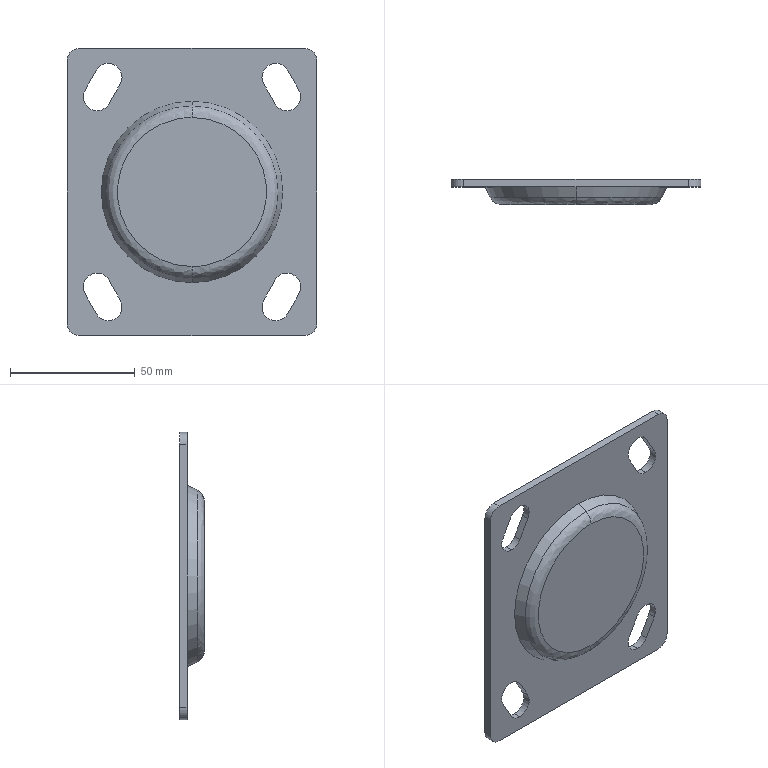Part | STEP file | _CEL21-100-P-002 | 1 solid | 41 faces | box 100 x 10 x 115 mm | volume 55123 mm3 | cylinder 20 | plane 17 | spline 2 | cone 2 | commonest cylinder face diameters 11 x12 10 x4 25 x2 66.667 x2
STEP:
#1=CARTESIAN_POINT('',(0.,84.,-60.815));
#2=VERTEX_POINT('',#1);
#3=CARTESIAN_POINT('',(0.,84.,-1.185));
#4=VERTEX_POINT('',#3);
#5=CARTESIAN_POINT('',(0.,84.,-60.815));
#6=CARTESIAN_POINT('',(-59.629,84.,-60.815));
#7=CARTESIAN_POINT('',(-59.629,84.,-1.185));
#8=CARTESIAN_POINT('',(0.,84.,-1.185));
#9=(BOUNDED_CURVE()B_SPLINE_CURVE(3,(#5,#6,#7,#8),.UNSPECIFIED.,.F.,.F.)B_SPLINE_CURVE_WITH_KNOTS((4,4),(0.,0.5),.UNSPECIFIED.)CURVE()GEOMETRIC_REPRESENTATION_ITEM()RATIONAL_B_SPLINE_CURVE((1.,0.3333,0.3333,1.))REPRESENTATION_ITEM(''));
#10=EDGE_CURVE('',#2,#4,#9,.T.);
#11=ORIENTED_EDGE('',*,*,#10,.T.);
#12=CARTESIAN_POINT('',(0.,86.887,3.346));
#13=VERTEX_POINT('',#12);
#14=CARTESIAN_POINT('',(0.,89.,-1.185));
#15=DIRECTION('',(-1.,0.,0.));
#16=DIRECTION('',(0.,0.,1.));
#17=AXIS2_PLACEMENT_3D('',#14,#15,#16);
#18=CIRCLE('',#17,5.);
#19=EDGE_CURVE('',#4,#13,#18,.T.);
#20=ORIENTED_EDGE('',*,*,#19,.T.);
#21=CARTESIAN_POINT('',(0.,86.887,-65.346));
#22=VERTEX_POINT('',#21);
#23=CARTESIAN_POINT('',(0.,86.887,-31.));
#24=DIRECTION('',(0.,1.,0.));
#25=DIRECTION('',(0.,0.,1.));
#26=AXIS2_PLACEMENT_3D('',#23,#24,#25);
#27=CIRCLE('',#26,34.346);
#28=EDGE_CURVE('',#22,#13,#27,.T.);
#29=ORIENTED_EDGE('',*,*,#28,.F.);
#30=CARTESIAN_POINT('',(0.,89.,-60.815));
#31=DIRECTION('',(1.,0.,0.));
#32=DIRECTION('',(0.,0.,-1.));
#33=AXIS2_PLACEMENT_3D('',#30,#31,#32);
#34=CIRCLE('',#33,5.);
#35=EDGE_CURVE('',#2,#22,#34,.T.);
#36=ORIENTED_EDGE('',*,*,#35,.F.);
#37=EDGE_LOOP('',(#11,#20,#29,#36));
#38=FACE_OUTER_BOUND('',#37,.T.);
#39=CARTESIAN_POINT('',(0.,84.,-1.185));
#40=CARTESIAN_POINT('',(-59.629,84.,-1.185));
#41=CARTESIAN_POINT('',(-59.629,84.,-60.815));
#42=CARTESIAN_POINT('',(0.,84.,-60.815));
#43=CARTESIAN_POINT('',(0.,84.,0.8144));
#44=CARTESIAN_POINT('',(-63.629,84.,0.8144));
#45=CARTESIAN_POINT('',(-63.629,84.,-62.814));
#46=CARTESIAN_POINT('',(0.,84.,-62.814));
#47=CARTESIAN_POINT('',(0.,85.074,2.501));
#48=CARTESIAN_POINT('',(-67.002,85.074,2.501));
#49=CARTESIAN_POINT('',(-67.002,85.074,-64.501));
#50=CARTESIAN_POINT('',(0.,85.074,-64.501));
#51=CARTESIAN_POINT('',(0.,86.887,3.346));
#52=CARTESIAN_POINT('',(-68.692,86.887,3.346));
#53=CARTESIAN_POINT('',(-68.692,86.887,-65.346));
#54=CARTESIAN_POINT('',(0.,86.887,-65.346));
#55=(BOUNDED_SURFACE()B_SPLINE_SURFACE(3,3,((#39,#40,#41,#42),(#43,#44,#45,#46),(#47,#48,#49,#50),(#51,#52,#53,#54)),.UNSPECIFIED.,.F.,.F.,.F.)B_SPLINE_SURFACE_WITH_KNOTS((4,4),(4,4),(0.,1.),(0.,1.),.UNSPECIFIED.)GEOMETRIC_REPRESENTATION_ITEM()RATIONAL_B_SPLINE_SURFACE(((1.,0.3333,0.3333,1.),(0.8956,0.2985,0.2985,0.8956),(0.8956,0.2985,0.2985,0.8956),(1.,0.3333,0.3333,1.)))REPRESENTATION_ITEM('')SURFACE());
#56=ADVANCED_FACE('',(#38),#55,.T.);
#57=CARTESIAN_POINT('',(33.5,94.,-82.5));
#58=VERTEX_POINT('',#57);
#59=CARTESIAN_POINT('',(38.294,94.,-79.696));
#60=VERTEX_POINT('',#59);
#61=CARTESIAN_POINT('',(33.5,94.,-77.));
#62=DIRECTION('',(0.,-1.,0.));
#63=DIRECTION('',(0.,0.,-1.));
#64=AXIS2_PLACEMENT_3D('',#61,#62,#63);
#65=CIRCLE('',#64,5.5);
#66=EDGE_CURVE('',#58,#60,#65,.T.);
#67=ORIENTED_EDGE('',*,*,#66,.F.);
#68=CARTESIAN_POINT('',(33.5,91.,-82.5));
#69=VERTEX_POINT('',#68);
#70=CARTESIAN_POINT('',(33.5,91.,-82.5));
#71=DIRECTION('',(0.,-1.,0.));
#72=VECTOR('',#71,1000.);
#73=LINE('',#70,#72);
#74=EDGE_CURVE('',#58,#69,#73,.T.);
#75=ORIENTED_EDGE('',*,*,#74,.T.);
#76=CARTESIAN_POINT('',(38.294,91.,-79.696));
#77=VERTEX_POINT('',#76);
#78=CARTESIAN_POINT('',(33.5,91.,-77.));
#79=DIRECTION('',(0.,1.,0.));
#80=DIRECTION('',(0.,0.,-1.));
#81=AXIS2_PLACEMENT_3D('',#78,#79,#80);
#82=CIRCLE('',#81,5.5);
#83=EDGE_CURVE('',#77,#69,#82,.T.);
#84=ORIENTED_EDGE('',*,*,#83,.F.);
#85=CARTESIAN_POINT('',(38.294,91.,-79.696));
#86=DIRECTION('',(0.,-1.,0.));
#87=VECTOR('',#86,1000.);
#88=LINE('',#85,#87);
#89=EDGE_CURVE('',#60,#77,#88,.T.);
#90=ORIENTED_EDGE('',*,*,#89,.F.);
#91=EDGE_LOOP('',(#67,#75,#84,#90));
#92=FACE_OUTER_BOUND('',#91,.T.);
#93=CARTESIAN_POINT('',(33.5,91.,-77.));
#94=DIRECTION('',(0.,-1.,0.));
#95=DIRECTION('',(0.,0.,-1.));
#96=AXIS2_PLACEMENT_3D('',#93,#94,#95);
#97=CYLINDRICAL_SURFACE('',#96,5.5);
#98=ADVANCED_FACE('',(#92),#97,.F.);
#99=CARTESIAN_POINT('',(38.,94.,1.5));
#100=VERTEX_POINT('',#99);
#101=CARTESIAN_POINT('',(42.794,94.,9.696));
#102=VERTEX_POINT('',#101);
#103=CARTESIAN_POINT('',(38.,94.,7.));
#104=DIRECTION('',(0.,-1.,0.));
#105=DIRECTION('',(0.,0.,-1.));
#106=AXIS2_PLACEMENT_3D('',#103,#104,#105);
#107=CIRCLE('',#106,5.5);
#108=EDGE_CURVE('',#100,#102,#107,.T.);
#109=ORIENTED_EDGE('',*,*,#108,.F.);
#110=CARTESIAN_POINT('',(38.,91.,1.5));
#111=VERTEX_POINT('',#110);
#112=CARTESIAN_POINT('',(38.,91.,1.5));
#113=DIRECTION('',(0.,-1.,0.));
#114=VECTOR('',#113,1000.);
#115=LINE('',#112,#114);
#116=EDGE_CURVE('',#100,#111,#115,.T.);
#117=ORIENTED_EDGE('',*,*,#116,.T.);
#118=CARTESIAN_POINT('',(42.794,91.,9.696));
#119=VERTEX_POINT('',#118);
#120=CARTESIAN_POINT('',(38.,91.,7.));
#121=DIRECTION('',(0.,1.,0.));
#122=DIRECTION('',(0.,0.,-1.));
#123=AXIS2_PLACEMENT_3D('',#120,#121,#122);
#124=CIRCLE('',#123,5.5);
#125=EDGE_CURVE('',#119,#111,#124,.T.);
#126=ORIENTED_EDGE('',*,*,#125,.F.);
#127=CARTESIAN_POINT('',(42.794,91.,9.696));
#128=DIRECTION('',(0.,1.,0.));
#129=VECTOR('',#128,1000.);
#130=LINE('',#127,#129);
#131=EDGE_CURVE('',#119,#102,#130,.T.);
#132=ORIENTED_EDGE('',*,*,#131,.T.);
#133=EDGE_LOOP('',(#109,#117,#126,#132));
#134=FACE_OUTER_BOUND('',#133,.T.);
#135=CARTESIAN_POINT('',(38.,91.,7.));
#136=DIRECTION('',(0.,-1.,0.));
#137=DIRECTION('',(0.,0.,-1.));
#138=AXIS2_PLACEMENT_3D('',#135,#136,#137);
#139=CYLINDRICAL_SURFACE('',#138,5.5);
#140=ADVANCED_FACE('',(#134),#139,.F.);
#141=CARTESIAN_POINT('',(-33.5,94.,-82.5));
#142=VERTEX_POINT('',#141);
#143=CARTESIAN_POINT('',(-28.706,94.,-74.304));
#144=VERTEX_POINT('',#143);
#145=CARTESIAN_POINT('',(-33.5,94.,-77.));
#146=DIRECTION('',(0.,-1.,0.));
#147=DIRECTION('',(0.,0.,-1.));
#148=AXIS2_PLACEMENT_3D('',#145,#146,#147);
#149=CIRCLE('',#148,5.5);
#150=EDGE_CURVE('',#142,#144,#149,.T.);
#151=ORIENTED_EDGE('',*,*,#150,.F.);
#152=CARTESIAN_POINT('',(-33.5,91.,-82.5));
#153=VERTEX_POINT('',#152);
#154=CARTESIAN_POINT('',(-33.5,91.,-82.5));
#155=DIRECTION('',(0.,-1.,0.));
#156=VECTOR('',#155,1000.);
#157=LINE('',#154,#156);
#158=EDGE_CURVE('',#142,#153,#157,.T.);
#159=ORIENTED_EDGE('',*,*,#158,.T.);
#160=CARTESIAN_POINT('',(-28.706,91.,-74.304));
#161=VERTEX_POINT('',#160);
#162=CARTESIAN_POINT('',(-33.5,91.,-77.));
#163=DIRECTION('',(0.,1.,0.));
#164=DIRECTION('',(0.,0.,-1.));
#165=AXIS2_PLACEMENT_3D('',#162,#163,#164);
#166=CIRCLE('',#165,5.5);
#167=EDGE_CURVE('',#161,#153,#166,.T.);
#168=ORIENTED_EDGE('',*,*,#167,.F.);
#169=CARTESIAN_POINT('',(-28.706,91.,-74.304));
#170=DIRECTION('',(0.,1.,0.));
#171=VECTOR('',#170,1000.);
#172=LINE('',#169,#171);
#173=EDGE_CURVE('',#161,#144,#172,.T.);
#174=ORIENTED_EDGE('',*,*,#173,.T.);
#175=EDGE_LOOP('',(#151,#159,#168,#174));
#176=FACE_OUTER_BOUND('',#175,.T.);
#177=CARTESIAN_POINT('',(-33.5,91.,-77.));
#178=DIRECTION('',(0.,-1.,0.));
#179=DIRECTION('',(0.,0.,-1.));
#180=AXIS2_PLACEMENT_3D('',#177,#178,#179);
#181=CYLINDRICAL_SURFACE('',#180,5.5);
#182=ADVANCED_FACE('',(#176),#181,.F.);
#183=CARTESIAN_POINT('',(-38.,94.,1.5));
#184=VERTEX_POINT('',#183);
#185=CARTESIAN_POINT('',(-33.206,94.,4.304));
#186=VERTEX_POINT('',#185);
#187=CARTESIAN_POINT('',(-38.,94.,7.));
#188=DIRECTION('',(0.,-1.,0.));
#189=DIRECTION('',(0.,0.,-1.));
#190=AXIS2_PLACEMENT_3D('',#187,#188,#189);
#191=CIRCLE('',#190,5.5);
#192=EDGE_CURVE('',#184,#186,#191,.T.);
#193=ORIENTED_EDGE('',*,*,#192,.F.);
#194=CARTESIAN_POINT('',(-38.,91.,1.5));
#195=VERTEX_POINT('',#194);
#196=CARTESIAN_POINT('',(-38.,91.,1.5));
#197=DIRECTION('',(0.,-1.,0.));
#198=VECTOR('',#197,1000.);
#199=LINE('',#196,#198);
#200=EDGE_CURVE('',#184,#195,#199,.T.);
#201=ORIENTED_EDGE('',*,*,#200,.T.);
#202=CARTESIAN_POINT('',(-33.206,91.,4.304));
#203=VERTEX_POINT('',#202);
#204=CARTESIAN_POINT('',(-38.,91.,7.));
#205=DIRECTION('',(0.,1.,0.));
#206=DIRECTION('',(0.,0.,-1.));
#207=AXIS2_PLACEMENT_3D('',#204,#205,#206);
#208=CIRCLE('',#207,5.5);
#209=EDGE_CURVE('',#203,#195,#208,.T.);
#210=ORIENTED_EDGE('',*,*,#209,.F.);
#211=CARTESIAN_POINT('',(-33.206,91.,4.304));
#212=DIRECTION('',(0.,-1.,0.));
#213=VECTOR('',#212,1000.);
#214=LINE('',#211,#213);
#215=EDGE_CURVE('',#186,#203,#214,.T.);
#216=ORIENTED_EDGE('',*,*,#215,.F.);
#217=EDGE_LOOP('',(#193,#201,#210,#216));
#218=FACE_OUTER_BOUND('',#217,.T.);
#219=CARTESIAN_POINT('',(-38.,91.,7.));
#220=DIRECTION('',(0.,-1.,0.));
#221=DIRECTION('',(0.,0.,-1.));
#222=AXIS2_PLACEMENT_3D('',#219,#220,#221);
#223=CYLINDRICAL_SURFACE('',#222,5.5);
#224=ADVANCED_FACE('',(#218),#223,.F.);
#225=CARTESIAN_POINT('',(0.,94.,2.333));
#226=VERTEX_POINT('',#225);
#227=CARTESIAN_POINT('',(0.,94.,-64.333));
#228=VERTEX_POINT('',#227);
#229=CARTESIAN_POINT('',(0.,94.,-31.));
#230=DIRECTION('',(0.,-1.,0.));
#231=DIRECTION('',(0.,0.,-1.));
#232=AXIS2_PLACEMENT_3D('',#229,#230,#231);
#233=CIRCLE('',#232,33.333);
#234=EDGE_CURVE('',#226,#228,#233,.T.);
#235=ORIENTED_EDGE('',*,*,#234,.F.);
#236=CARTESIAN_POINT('',(0.,93.,2.333));
#237=VERTEX_POINT('',#236);
#238=CARTESIAN_POINT('',(0.,93.,2.333));
#239=DIRECTION('',(0.,-1.,0.));
#240=VECTOR('',#239,1000.);
#241=LINE('',#238,#240);
#242=EDGE_CURVE('',#226,#237,#241,.T.);
#243=ORIENTED_EDGE('',*,*,#242,.T.);
#244=CARTESIAN_POINT('',(0.,93.,-64.333));
#245=VERTEX_POINT('',#244);
#246=CARTESIAN_POINT('',(0.,93.,-31.));
#247=DIRECTION('',(0.,1.,0.));
#248=DIRECTION('',(0.,0.,-1.));
#249=AXIS2_PLACEMENT_3D('',#246,#247,#248);
#250=CIRCLE('',#249,33.333);
#251=EDGE_CURVE('',#245,#237,#250,.T.);
#252=ORIENTED_EDGE('',*,*,#251,.F.);
#253=CARTESIAN_POINT('',(0.,93.,-64.333));
#254=DIRECTION('',(0.,-1.,0.));
#255=VECTOR('',#254,1000.);
#256=LINE('',#253,#255);
#257=EDGE_CURVE('',#228,#245,#256,.T.);
#258=ORIENTED_EDGE('',*,*,#257,.F.);
#259=EDGE_LOOP('',(#235,#243,#252,#258));
#260=FACE_OUTER_BOUND('',#259,.T.);
#261=CARTESIAN_POINT('',(0.,93.,-31.));
#262=DIRECTION('',(0.,-1.,0.));
#263=DIRECTION('',(0.,0.,-1.));
#264=AXIS2_PLACEMENT_3D('',#261,#262,#263);
#265=CYLINDRICAL_SURFACE('',#264,33.333);
#266=ADVANCED_FACE('',(#260),#265,.F.);
#267=CARTESIAN_POINT('',(0.,86.887,-31.));
#268=DIRECTION('',(0.,1.,0.));
#269=DIRECTION('',(0.,0.,1.));
#270=AXIS2_PLACEMENT_3D('',#267,#268,#269);
#271=CIRCLE('',#270,34.346);
#272=EDGE_CURVE('',#13,#22,#271,.T.);
#273=ORIENTED_EDGE('',*,*,#272,.T.);
#274=CARTESIAN_POINT('',(0.,91.,-67.264));
#275=VERTEX_POINT('',#274);
#276=CARTESIAN_POINT('',(0.,91.,-67.264));
#277=DIRECTION('',(0.,0.9063,-0.4226));
#278=VECTOR('',#277,1000.);
#279=LINE('',#276,#278);
#280=EDGE_CURVE('',#22,#275,#279,.T.);
#281=ORIENTED_EDGE('',*,*,#280,.T.);
#282=CARTESIAN_POINT('',(0.,91.,5.264));
#283=VERTEX_POINT('',#282);
#284=CARTESIAN_POINT('',(0.,91.,-31.));
#285=DIRECTION('',(0.,-1.,0.));
#286=DIRECTION('',(0.,0.,1.));
#287=AXIS2_PLACEMENT_3D('',#284,#285,#286);
#288=CIRCLE('',#287,36.264);
#289=EDGE_CURVE('',#275,#283,#288,.T.);
#290=ORIENTED_EDGE('',*,*,#289,.T.);
#291=CARTESIAN_POINT('',(0.,91.,5.264));
#292=DIRECTION('',(0.,0.9063,0.4226));
#293=VECTOR('',#292,1000.);
#294=LINE('',#291,#293);
#295=EDGE_CURVE('',#13,#283,#294,.T.);
#296=ORIENTED_EDGE('',*,*,#295,.F.);
#297=EDGE_LOOP('',(#273,#281,#290,#296));
#298=FACE_OUTER_BOUND('',#297,.T.);
#299=CARTESIAN_POINT('',(0.,91.,-31.));
#300=DIRECTION('',(0.,1.,0.));
#301=DIRECTION('',(0.,0.,1.));
#302=AXIS2_PLACEMENT_3D('',#299,#300,#301);
#303=CONICAL_SURFACE('',#302,36.264,0.4363);
#304=ADVANCED_FACE('',(#298),#303,.T.);
#305=CARTESIAN_POINT('',(0.,94.,-43.5));
#306=VERTEX_POINT('',#305);
#307=CARTESIAN_POINT('',(0.,94.,-18.5));
#308=VERTEX_POINT('',#307);
#309=CARTESIAN_POINT('',(0.,94.,-31.));
#310=DIRECTION('',(0.,-1.,0.));
#311=DIRECTION('',(0.,0.,-1.));
#312=AXIS2_PLACEMENT_3D('',#309,#310,#311);
#313=CIRCLE('',#312,12.5);
#314=EDGE_CURVE('',#306,#308,#313,.T.);
#315=ORIENTED_EDGE('',*,*,#314,.T.);
#316=CARTESIAN_POINT('',(0.,93.,-18.5));
#317=VERTEX_POINT('',#316);
#318=CARTESIAN_POINT('',(0.,93.,-18.5));
#319=DIRECTION('',(0.,-1.,0.));
#320=VECTOR('',#319,1000.);
#321=LINE('',#318,#320);
#322=EDGE_CURVE('',#308,#317,#321,.T.);
#323=ORIENTED_EDGE('',*,*,#322,.T.);
#324=CARTESIAN_POINT('',(0.,93.,-43.5));
#325=VERTEX_POINT('',#324);
#326=CARTESIAN_POINT('',(0.,93.,-31.));
#327=DIRECTION('',(0.,-1.,0.));
#328=DIRECTION('',(0.,0.,-1.));
#329=AXIS2_PLACEMENT_3D('',#326,#327,#328);
#330=CIRCLE('',#329,12.5);
#331=EDGE_CURVE('',#325,#317,#330,.T.);
#332=ORIENTED_EDGE('',*,*,#331,.F.);
#333=CARTESIAN_POINT('',(0.,93.,-43.5));
#334=DIRECTION('',(0.,-1.,0.));
#335=VECTOR('',#334,1000.);
#336=LINE('',#333,#335);
#337=EDGE_CURVE('',#306,#325,#336,.T.);
#338=ORIENTED_EDGE('',*,*,#337,.F.);
#339=EDGE_LOOP('',(#315,#323,#332,#338));
#340=FACE_OUTER_BOUND('',#339,.T.);
#341=CARTESIAN_POINT('',(0.,93.,-31.));
#342=DIRECTION('',(0.,-1.,0.));
#343=DIRECTION('',(0.,0.,-1.));
#344=AXIS2_PLACEMENT_3D('',#341,#342,#343);
#345=CYLINDRICAL_SURFACE('',#344,12.5);
#346=ADVANCED_FACE('',(#340),#345,.T.);
#347=CARTESIAN_POINT('',(50.,94.,-83.5));
#348=VERTEX_POINT('',#347);
#349=CARTESIAN_POINT('',(45.,94.,-88.5));
#350=VERTEX_POINT('',#349);
#351=CARTESIAN_POINT('',(45.,94.,-83.5));
#352=DIRECTION('',(0.,1.,0.));
#353=DIRECTION('',(0.,0.,-1.));
#354=AXIS2_PLACEMENT_3D('',#351,#352,#353);
#355=CIRCLE('',#354,5.);
#356=EDGE_CURVE('',#348,#350,#355,.T.);
#357=ORIENTED_EDGE('',*,*,#356,.T.);
#358=CARTESIAN_POINT('',(-45.,94.,-88.5));
#359=VERTEX_POINT('',#358);
#360=CARTESIAN_POINT('',(-45.,94.,-88.5));
#361=DIRECTION('',(-1.,0.,0.));
#362=VECTOR('',#361,1000.);
#363=LINE('',#360,#362);
#364=EDGE_CURVE('',#350,#359,#363,.T.);
#365=ORIENTED_EDGE('',*,*,#364,.T.);
#366=CARTESIAN_POINT('',(-50.,94.,-83.5));
#367=VERTEX_POINT('',#366);
#368=CARTESIAN_POINT('',(-45.,94.,-83.5));
#369=DIRECTION('',(0.,1.,0.));
#370=DIRECTION('',(0.,0.,-1.));
#371=AXIS2_PLACEMENT_3D('',#368,#369,#370);
#372=CIRCLE('',#371,5.);
#373=EDGE_CURVE('',#359,#367,#372,.T.);
#374=ORIENTED_EDGE('',*,*,#373,.T.);
#375=CARTESIAN_POINT('',(-50.,94.,21.5));
#376=VERTEX_POINT('',#375);
#377=CARTESIAN_POINT('',(-50.,94.,-83.5));
#378=DIRECTION('',(0.,0.,1.));
#379=VECTOR('',#378,1000.);
#380=LINE('',#377,#379);
#381=EDGE_CURVE('',#367,#376,#380,.T.);
#382=ORIENTED_EDGE('',*,*,#381,.T.);
#383=CARTESIAN_POINT('',(-45.,94.,26.5));
#384=VERTEX_POINT('',#383);
#385=CARTESIAN_POINT('',(-45.,94.,21.5));
#386=DIRECTION('',(0.,1.,0.));
#387=DIRECTION('',(0.,0.,-1.));
#388=AXIS2_PLACEMENT_3D('',#385,#386,#387);
#389=CIRCLE('',#388,5.);
#390=EDGE_CURVE('',#376,#384,#389,.T.);
#391=ORIENTED_EDGE('',*,*,#390,.T.);
#392=CARTESIAN_POINT('',(45.,94.,26.5));
#393=VERTEX_POINT('',#392);
#394=CARTESIAN_POINT('',(-45.,94.,26.5));
#395=DIRECTION('',(1.,0.,0.));
#396=VECTOR('',#395,1000.);
#397=LINE('',#394,#396);
#398=EDGE_CURVE('',#384,#393,#397,.T.);
#399=ORIENTED_EDGE('',*,*,#398,.T.);
#400=CARTESIAN_POINT('',(50.,94.,21.5));
#401=VERTEX_POINT('',#400);
#402=CARTESIAN_POINT('',(45.,94.,21.5));
#403=DIRECTION('',(0.,1.,0.));
#404=DIRECTION('',(0.,0.,-1.));
#405=AXIS2_PLACEMENT_3D('',#402,#403,#404);
#406=CIRCLE('',#405,5.);
#407=EDGE_CURVE('',#393,#401,#406,.T.);
#408=ORIENTED_EDGE('',*,*,#407,.T.);
#409=CARTESIAN_POINT('',(50.,94.,-83.5));
#410=DIRECTION('',(0.,0.,-1.));
#411=VECTOR('',#410,1000.);
#412=LINE('',#409,#411);
#413=EDGE_CURVE('',#401,#348,#412,.T.);
#414=ORIENTED_EDGE('',*,*,#413,.T.);
#415=EDGE_LOOP('',(#357,#365,#374,#382,#391,#399,#408,#414));
#416=FACE_OUTER_BOUND('',#415,.T.);
#417=CARTESIAN_POINT('',(33.206,94.,-66.304));
#418=VERTEX_POINT('',#417);
#419=CARTESIAN_POINT('',(28.706,94.,-74.304));
#420=VERTEX_POINT('',#419);
#421=CARTESIAN_POINT('',(33.206,94.,-66.304));
#422=DIRECTION('',(-0.4903,0.,-0.8716));
#423=VECTOR('',#422,1000.);
#424=LINE('',#421,#423);
#425=EDGE_CURVE('',#418,#420,#424,.T.);
#426=ORIENTED_EDGE('',*,*,#425,.T.);
#427=CARTESIAN_POINT('',(33.5,94.,-77.));
#428=DIRECTION('',(0.,-1.,0.));
#429=DIRECTION('',(0.,0.,-1.));
#430=AXIS2_PLACEMENT_3D('',#427,#428,#429);
#431=CIRCLE('',#430,5.5);
#432=EDGE_CURVE('',#420,#58,#431,.T.);
#433=ORIENTED_EDGE('',*,*,#432,.T.);
#434=ORIENTED_EDGE('',*,*,#66,.T.);
#435=CARTESIAN_POINT('',(42.794,94.,-71.696));
#436=VERTEX_POINT('',#435);
#437=CARTESIAN_POINT('',(38.294,94.,-79.696));
#438=DIRECTION('',(0.4903,0.,0.8716));
#439=VECTOR('',#438,1000.);
#440=LINE('',#437,#439);
#441=EDGE_CURVE('',#60,#436,#440,.T.);
#442=ORIENTED_EDGE('',*,*,#441,.T.);
#443=CARTESIAN_POINT('',(38.,94.,-69.));
#444=DIRECTION('',(0.,-1.,0.));
#445=DIRECTION('',(0.,0.,-1.));
#446=AXIS2_PLACEMENT_3D('',#443,#444,#445);
#447=CIRCLE('',#446,5.5);
#448=EDGE_CURVE('',#436,#418,#447,.T.);
#449=ORIENTED_EDGE('',*,*,#448,.T.);
#450=EDGE_LOOP('',(#426,#433,#434,#442,#449));
#451=FACE_BOUND('',#450,.T.);
#452=CARTESIAN_POINT('',(38.294,94.,17.696));
#453=VERTEX_POINT('',#452);
#454=CARTESIAN_POINT('',(42.794,94.,9.696));
#455=DIRECTION('',(-0.4903,0.,0.8716));
#456=VECTOR('',#455,1000.);
#457=LINE('',#454,#456);
#458=EDGE_CURVE('',#102,#453,#457,.T.);
#459=ORIENTED_EDGE('',*,*,#458,.T.);
#460=CARTESIAN_POINT('',(28.706,94.,12.304));
#461=VERTEX_POINT('',#460);
#462=CARTESIAN_POINT('',(33.5,94.,15.));
#463=DIRECTION('',(0.,-1.,0.));
#464=DIRECTION('',(0.,0.,-1.));
#465=AXIS2_PLACEMENT_3D('',#462,#463,#464);
#466=CIRCLE('',#465,5.5);
#467=EDGE_CURVE('',#453,#461,#466,.T.);
#468=ORIENTED_EDGE('',*,*,#467,.T.);
#469=CARTESIAN_POINT('',(33.206,94.,4.304));
#470=VERTEX_POINT('',#469);
#471=CARTESIAN_POINT('',(28.706,94.,12.304));
#472=DIRECTION('',(0.4903,0.,-0.8716));
#473=VECTOR('',#472,1000.);
#474=LINE('',#471,#473);
#475=EDGE_CURVE('',#461,#470,#474,.T.);
#476=ORIENTED_EDGE('',*,*,#475,.T.);
#477=CARTESIAN_POINT('',(38.,94.,7.));
#478=DIRECTION('',(0.,-1.,0.));
#479=DIRECTION('',(0.,0.,-1.));
#480=AXIS2_PLACEMENT_3D('',#477,#478,#479);
#481=CIRCLE('',#480,5.5);
#482=EDGE_CURVE('',#470,#100,#481,.T.);
#483=ORIENTED_EDGE('',*,*,#482,.T.);
#484=ORIENTED_EDGE('',*,*,#108,.T.);
#485=EDGE_LOOP('',(#459,#468,#476,#483,#484));
#486=FACE_BOUND('',#485,.T.);
#487=CARTESIAN_POINT('',(-33.206,94.,-66.304));
#488=VERTEX_POINT('',#487);
#489=CARTESIAN_POINT('',(-28.706,94.,-74.304));
#490=DIRECTION('',(-0.4903,0.,0.8716));
#491=VECTOR('',#490,1000.);
#492=LINE('',#489,#491);
#493=EDGE_CURVE('',#144,#488,#492,.T.);
#494=ORIENTED_EDGE('',*,*,#493,.T.);
#495=CARTESIAN_POINT('',(-42.794,94.,-71.696));
#496=VERTEX_POINT('',#495);
#497=CARTESIAN_POINT('',(-38.,94.,-69.));
#498=DIRECTION('',(0.,-1.,0.));
#499=DIRECTION('',(0.,0.,-1.));
#500=AXIS2_PLACEMENT_3D('',#497,#498,#499);
#501=CIRCLE('',#500,5.5);
#502=EDGE_CURVE('',#488,#496,#501,.T.);
#503=ORIENTED_EDGE('',*,*,#502,.T.);
#504=CARTESIAN_POINT('',(-38.294,94.,-79.696));
#505=VERTEX_POINT('',#504);
#506=CARTESIAN_POINT('',(-42.794,94.,-71.696));
#507=DIRECTION('',(0.4903,0.,-0.8716));
#508=VECTOR('',#507,1000.);
#509=LINE('',#506,#508);
#510=EDGE_CURVE('',#496,#505,#509,.T.);
#511=ORIENTED_EDGE('',*,*,#510,.T.);
#512=CARTESIAN_POINT('',(-33.5,94.,-77.));
#513=DIRECTION('',(0.,-1.,0.));
#514=DIRECTION('',(0.,0.,-1.));
#515=AXIS2_PLACEMENT_3D('',#512,#513,#514);
#516=CIRCLE('',#515,5.5);
#517=EDGE_CURVE('',#505,#142,#516,.T.);
#518=ORIENTED_EDGE('',*,*,#517,.T.);
#519=ORIENTED_EDGE('',*,*,#150,.T.);
#520=EDGE_LOOP('',(#494,#503,#511,#518,#519));
#521=FACE_BOUND('',#520,.T.);
#522=CARTESIAN_POINT('',(-38.294,94.,17.696));
#523=VERTEX_POINT('',#522);
#524=CARTESIAN_POINT('',(-42.794,94.,9.696));
#525=VERTEX_POINT('',#524);
#526=CARTESIAN_POINT('',(-38.294,94.,17.696));
#527=DIRECTION('',(-0.4903,0.,-0.8716));
#528=VECTOR('',#527,1000.);
#529=LINE('',#526,#528);
#530=EDGE_CURVE('',#523,#525,#529,.T.);
#531=ORIENTED_EDGE('',*,*,#530,.T.);
#532=CARTESIAN_POINT('',(-38.,94.,7.));
#533=DIRECTION('',(0.,-1.,0.));
#534=DIRECTION('',(0.,0.,-1.));
#535=AXIS2_PLACEMENT_3D('',#532,#533,#534);
#536=CIRCLE('',#535,5.5);
#537=EDGE_CURVE('',#525,#184,#536,.T.);
#538=ORIENTED_EDGE('',*,*,#537,.T.);
#539=ORIENTED_EDGE('',*,*,#192,.T.);
#540=CARTESIAN_POINT('',(-28.706,94.,12.304));
#541=VERTEX_POINT('',#540);
#542=CARTESIAN_POINT('',(-33.206,94.,4.304));
#543=DIRECTION('',(0.4903,0.,0.8716));
#544=VECTOR('',#543,1000.);
#545=LINE('',#542,#544);
#546=EDGE_CURVE('',#186,#541,#545,.T.);
#547=ORIENTED_EDGE('',*,*,#546,.T.);
#548=CARTESIAN_POINT('',(-33.5,94.,15.));
#549=DIRECTION('',(0.,-1.,0.));
#550=DIRECTION('',(0.,0.,-1.));
#551=AXIS2_PLACEMENT_3D('',#548,#549,#550);
#552=CIRCLE('',#551,5.5);
#553=EDGE_CURVE('',#541,#523,#552,.T.);
#554=ORIENTED_EDGE('',*,*,#553,.T.);
#555=EDGE_LOOP('',(#531,#538,#539,#547,#554));
#556=FACE_BOUND('',#555,.T.);
#557=CARTESIAN_POINT('',(0.,94.,-31.));
#558=DIRECTION('',(0.,-1.,0.));
#559=DIRECTION('',(0.,0.,-1.));
#560=AXIS2_PLACEMENT_3D('',#557,#558,#559);
#561=CIRCLE('',#560,33.333);
#562=EDGE_CURVE('',#228,#226,#561,.T.);
#563=ORIENTED_EDGE('',*,*,#562,.T.);
#564=ORIENTED_EDGE('',*,*,#234,.T.);
#565=EDGE_LOOP('',(#563,#564));
#566=FACE_BOUND('',#565,.T.);
#567=CARTESIAN_POINT('',(-45.,94.,-83.5));
#568=DIRECTION('',(0.,1.,0.));
#569=DIRECTION('',(0.,0.,1.));
#570=AXIS2_PLACEMENT_3D('',#567,#568,#569);
#571=PLANE('',#570);
#572=ADVANCED_FACE('',(#416,#451,#486,#521,#556,#566),#571,.T.);
#573=CARTESIAN_POINT('',(45.,91.,-88.5));
#574=VERTEX_POINT('',#573);
#575=CARTESIAN_POINT('',(-45.,91.,-88.5));
#576=VERTEX_POINT('',#575);
#577=CARTESIAN_POINT('',(45.,91.,-88.5));
#578=DIRECTION('',(-1.,0.,0.));
#579=VECTOR('',#578,1000.);
#580=LINE('',#577,#579);
#581=EDGE_CURVE('',#574,#576,#580,.T.);
#582=ORIENTED_EDGE('',*,*,#581,.T.);
#583=CARTESIAN_POINT('',(-45.,91.,-88.5));
#584=DIRECTION('',(0.,1.,0.));
#585=VECTOR('',#584,1000.);
#586=LINE('',#583,#585);
#587=EDGE_CURVE('',#576,#359,#586,.T.);
#588=ORIENTED_EDGE('',*,*,#587,.T.);
#589=ORIENTED_EDGE('',*,*,#364,.F.);
#590=CARTESIAN_POINT('',(45.,91.,-88.5));
#591=DIRECTION('',(0.,-1.,0.));
#592=VECTOR('',#591,1000.);
#593=LINE('',#590,#592);
#594=EDGE_CURVE('',#350,#574,#593,.T.);
#595=ORIENTED_EDGE('',*,*,#594,.T.);
#596=EDGE_LOOP('',(#582,#588,#589,#595));
#597=FACE_OUTER_BOUND('',#596,.T.);
#598=CARTESIAN_POINT('',(45.,91.,-88.5));
#599=DIRECTION('',(0.,0.,-1.));
#600=DIRECTION('',(-1.,0.,0.));
#601=AXIS2_PLACEMENT_3D('',#598,#599,#600);
#602=PLANE('',#601);
#603=ADVANCED_FACE('',(#597),#602,.T.);
#604=CARTESIAN_POINT('',(50.,91.,-83.5));
#605=VERTEX_POINT('',#604);
#606=CARTESIAN_POINT('',(45.,91.,-83.5));
#607=DIRECTION('',(0.,1.,0.));
#608=DIRECTION('',(0.,0.,-1.));
#609=AXIS2_PLACEMENT_3D('',#606,#607,#608);
#610=CIRCLE('',#609,5.);
#611=EDGE_CURVE('',#605,#574,#610,.T.);
#612=ORIENTED_EDGE('',*,*,#611,.T.);
#613=ORIENTED_EDGE('',*,*,#594,.F.);
#614=ORIENTED_EDGE('',*,*,#356,.F.);
#615=CARTESIAN_POINT('',(50.,91.,-83.5));
#616=DIRECTION('',(0.,-1.,0.));
#617=VECTOR('',#616,1000.);
#618=LINE('',#615,#617);
#619=EDGE_CURVE('',#348,#605,#618,.T.);
#620=ORIENTED_EDGE('',*,*,#619,.T.);
#621=EDGE_LOOP('',(#612,#613,#614,#620));
#622=FACE_OUTER_BOUND('',#621,.T.);
#623=CARTESIAN_POINT('',(45.,91.,-83.5));
#624=DIRECTION('',(0.,-1.,0.));
#625=DIRECTION('',(0.,0.,-1.));
#626=AXIS2_PLACEMENT_3D('',#623,#624,#625);
#627=CYLINDRICAL_SURFACE('',#626,5.);
#628=ADVANCED_FACE('',(#622),#627,.T.);
#629=CARTESIAN_POINT('',(50.,91.,21.5));
#630=VERTEX_POINT('',#629);
#631=CARTESIAN_POINT('',(50.,91.,21.5));
#632=DIRECTION('',(0.,0.,-1.));
#633=VECTOR('',#632,1000.);
#634=LINE('',#631,#633);
#635=EDGE_CURVE('',#630,#605,#634,.T.);
#636=ORIENTED_EDGE('',*,*,#635,.T.);
#637=ORIENTED_EDGE('',*,*,#619,.F.);
#638=ORIENTED_EDGE('',*,*,#413,.F.);
#639=CARTESIAN_POINT('',(50.,91.,21.5));
#640=DIRECTION('',(0.,-1.,0.));
#641=VECTOR('',#640,1000.);
#642=LINE('',#639,#641);
#643=EDGE_CURVE('',#401,#630,#642,.T.);
#644=ORIENTED_EDGE('',*,*,#643,.T.);
#645=EDGE_LOOP('',(#636,#637,#638,#644));
#646=FACE_OUTER_BOUND('',#645,.T.);
#647=CARTESIAN_POINT('',(50.,91.,21.5));
#648=DIRECTION('',(1.,0.,0.));
#649=DIRECTION('',(0.,0.,-1.));
#650=AXIS2_PLACEMENT_3D('',#647,#648,#649);
#651=PLANE('',#650);
#652=ADVANCED_FACE('',(#646),#651,.T.);
#653=CARTESIAN_POINT('',(45.,91.,26.5));
#654=VERTEX_POINT('',#653);
#655=CARTESIAN_POINT('',(45.,91.,21.5));
#656=DIRECTION('',(0.,1.,0.));
#657=DIRECTION('',(0.,0.,-1.));
#658=AXIS2_PLACEMENT_3D('',#655,#656,#657);
#659=CIRCLE('',#658,5.);
#660=EDGE_CURVE('',#654,#630,#659,.T.);
#661=ORIENTED_EDGE('',*,*,#660,.T.);
#662=ORIENTED_EDGE('',*,*,#643,.F.);
#663=ORIENTED_EDGE('',*,*,#407,.F.);
#664=CARTESIAN_POINT('',(45.,91.,26.5));
#665=DIRECTION('',(0.,-1.,0.));
#666=VECTOR('',#665,1000.);
#667=LINE('',#664,#666);
#668=EDGE_CURVE('',#393,#654,#667,.T.);
#669=ORIENTED_EDGE('',*,*,#668,.T.);
#670=EDGE_LOOP('',(#661,#662,#663,#669));
#671=FACE_OUTER_BOUND('',#670,.T.);
#672=CARTESIAN_POINT('',(45.,91.,21.5));
#673=DIRECTION('',(0.,-1.,0.));
#674=DIRECTION('',(0.,0.,-1.));
#675=AXIS2_PLACEMENT_3D('',#672,#673,#674);
#676=CYLINDRICAL_SURFACE('',#675,5.);
#677=ADVANCED_FACE('',(#671),#676,.T.);
#678=CARTESIAN_POINT('',(-45.,91.,26.5));
#679=VERTEX_POINT('',#678);
#680=CARTESIAN_POINT('',(-45.,91.,26.5));
#681=DIRECTION('',(1.,0.,0.));
#682=VECTOR('',#681,1000.);
#683=LINE('',#680,#682);
#684=EDGE_CURVE('',#679,#654,#683,.T.);
#685=ORIENTED_EDGE('',*,*,#684,.T.);
#686=ORIENTED_EDGE('',*,*,#668,.F.);
#687=ORIENTED_EDGE('',*,*,#398,.F.);
#688=CARTESIAN_POINT('',(-45.,91.,26.5));
#689=DIRECTION('',(0.,-1.,0.));
#690=VECTOR('',#689,1000.);
#691=LINE('',#688,#690);
#692=EDGE_CURVE('',#384,#679,#691,.T.);
#693=ORIENTED_EDGE('',*,*,#692,.T.);
#694=EDGE_LOOP('',(#685,#686,#687,#693));
#695=FACE_OUTER_BOUND('',#694,.T.);
#696=CARTESIAN_POINT('',(-45.,91.,26.5));
#697=DIRECTION('',(0.,0.,1.));
#698=DIRECTION('',(1.,0.,0.));
#699=AXIS2_PLACEMENT_3D('',#696,#697,#698);
#700=PLANE('',#699);
#701=ADVANCED_FACE('',(#695),#700,.T.);
#702=CARTESIAN_POINT('',(-50.,91.,21.5));
#703=VERTEX_POINT('',#702);
#704=CARTESIAN_POINT('',(-45.,91.,21.5));
#705=DIRECTION('',(0.,1.,0.));
#706=DIRECTION('',(0.,0.,-1.));
#707=AXIS2_PLACEMENT_3D('',#704,#705,#706);
#708=CIRCLE('',#707,5.);
#709=EDGE_CURVE('',#703,#679,#708,.T.);
#710=ORIENTED_EDGE('',*,*,#709,.T.);
#711=ORIENTED_EDGE('',*,*,#692,.F.);
#712=ORIENTED_EDGE('',*,*,#390,.F.);
#713=CARTESIAN_POINT('',(-50.,91.,21.5));
#714=DIRECTION('',(0.,-1.,0.));
#715=VECTOR('',#714,1000.);
#716=LINE('',#713,#715);
#717=EDGE_CURVE('',#376,#703,#716,.T.);
#718=ORIENTED_EDGE('',*,*,#717,.T.);
#719=EDGE_LOOP('',(#710,#711,#712,#718));
#720=FACE_OUTER_BOUND('',#719,.T.);
#721=CARTESIAN_POINT('',(-45.,91.,21.5));
#722=DIRECTION('',(0.,-1.,0.));
#723=DIRECTION('',(0.,0.,-1.));
#724=AXIS2_PLACEMENT_3D('',#721,#722,#723);
#725=CYLINDRICAL_SURFACE('',#724,5.);
#726=ADVANCED_FACE('',(#720),#725,.T.);
#727=CARTESIAN_POINT('',(-50.,91.,-83.5));
#728=VERTEX_POINT('',#727);
#729=CARTESIAN_POINT('',(-50.,91.,-83.5));
#730=DIRECTION('',(0.,0.,1.));
#731=VECTOR('',#730,1000.);
#732=LINE('',#729,#731);
#733=EDGE_CURVE('',#728,#703,#732,.T.);
#734=ORIENTED_EDGE('',*,*,#733,.T.);
#735=ORIENTED_EDGE('',*,*,#717,.F.);
#736=ORIENTED_EDGE('',*,*,#381,.F.);
#737=CARTESIAN_POINT('',(-50.,91.,-83.5));
#738=DIRECTION('',(0.,-1.,0.));
#739=VECTOR('',#738,1000.);
#740=LINE('',#737,#739);
#741=EDGE_CURVE('',#367,#728,#740,.T.);
#742=ORIENTED_EDGE('',*,*,#741,.T.);
#743=EDGE_LOOP('',(#734,#735,#736,#742));
#744=FACE_OUTER_BOUND('',#743,.T.);
#745=CARTESIAN_POINT('',(-50.,91.,-83.5));
#746=DIRECTION('',(-1.,0.,0.));
#747=DIRECTION('',(0.,0.,1.));
#748=AXIS2_PLACEMENT_3D('',#745,#746,#747);
#749=PLANE('',#748);
#750=ADVANCED_FACE('',(#744),#749,.T.);
#751=CARTESIAN_POINT('',(-45.,91.,-83.5));
#752=DIRECTION('',(0.,1.,0.));
#753=DIRECTION('',(0.,0.,-1.));
#754=AXIS2_PLACEMENT_3D('',#751,#752,#753);
#755=CIRCLE('',#754,5.);
#756=EDGE_CURVE('',#576,#728,#755,.T.);
#757=ORIENTED_EDGE('',*,*,#756,.T.);
#758=ORIENTED_EDGE('',*,*,#741,.F.);
#759=ORIENTED_EDGE('',*,*,#373,.F.);
#760=ORIENTED_EDGE('',*,*,#587,.F.);
#761=EDGE_LOOP('',(#757,#758,#759,#760));
#762=FACE_OUTER_BOUND('',#761,.T.);
#763=CARTESIAN_POINT('',(-45.,91.,-83.5));
#764=DIRECTION('',(0.,-1.,0.));
#765=DIRECTION('',(0.,0.,-1.));
#766=AXIS2_PLACEMENT_3D('',#763,#764,#765);
#767=CYLINDRICAL_SURFACE('',#766,5.);
#768=ADVANCED_FACE('',(#762),#767,.T.);
#769=ORIENTED_EDGE('',*,*,#74,.F.);
#770=ORIENTED_EDGE('',*,*,#432,.F.);
#771=CARTESIAN_POINT('',(28.706,91.,-74.304));
#772=VERTEX_POINT('',#771);
#773=CARTESIAN_POINT('',(28.706,91.,-74.304));
#774=DIRECTION('',(0.,1.,0.));
#775=VECTOR('',#774,1000.);
#776=LINE('',#773,#775);
#777=EDGE_CURVE('',#772,#420,#776,.T.);
#778=ORIENTED_EDGE('',*,*,#777,.F.);
#779=CARTESIAN_POINT('',(33.5,91.,-77.));
#780=DIRECTION('',(0.,1.,0.));
#781=DIRECTION('',(0.,0.,-1.));
#782=AXIS2_PLACEMENT_3D('',#779,#780,#781);
#783=CIRCLE('',#782,5.5);
#784=EDGE_CURVE('',#69,#772,#783,.T.);
#785=ORIENTED_EDGE('',*,*,#784,.F.);
#786=EDGE_LOOP('',(#769,#770,#778,#785));
#787=FACE_OUTER_BOUND('',#786,.T.);
#788=CARTESIAN_POINT('',(33.5,91.,-77.));
#789=DIRECTION('',(0.,-1.,0.));
#790=DIRECTION('',(0.,0.,-1.));
#791=AXIS2_PLACEMENT_3D('',#788,#789,#790);
#792=CYLINDRICAL_SURFACE('',#791,5.5);
#793=ADVANCED_FACE('',(#787),#792,.F.);
#794=CARTESIAN_POINT('',(33.206,91.,-66.304));
#795=VERTEX_POINT('',#794);
#796=CARTESIAN_POINT('',(33.206,91.,-66.304));
#797=DIRECTION('',(0.,1.,0.));
#798=VECTOR('',#797,1000.);
#799=LINE('',#796,#798);
#800=EDGE_CURVE('',#795,#418,#799,.T.);
#801=ORIENTED_EDGE('',*,*,#800,.F.);
#802=CARTESIAN_POINT('',(28.706,91.,-74.304));
#803=DIRECTION('',(0.4903,0.,0.8716));
#804=VECTOR('',#803,1000.);
#805=LINE('',#802,#804);
#806=EDGE_CURVE('',#772,#795,#805,.T.);
#807=ORIENTED_EDGE('',*,*,#806,.F.);
#808=ORIENTED_EDGE('',*,*,#777,.T.);
#809=ORIENTED_EDGE('',*,*,#425,.F.);
#810=EDGE_LOOP('',(#801,#807,#808,#809));
#811=FACE_OUTER_BOUND('',#810,.T.);
#812=CARTESIAN_POINT('',(28.706,91.,-74.304));
#813=DIRECTION('',(-0.8716,0.,0.4903));
#814=DIRECTION('',(0.4903,0.,0.8716));
#815=AXIS2_PLACEMENT_3D('',#812,#813,#814);
#816=PLANE('',#815);
#817=ADVANCED_FACE('',(#811),#816,.F.);
#818=CARTESIAN_POINT('',(42.794,91.,-71.696));
#819=VERTEX_POINT('',#818);
#820=CARTESIAN_POINT('',(42.794,91.,-71.696));
#821=DIRECTION('',(0.,1.,0.));
#822=VECTOR('',#821,1000.);
#823=LINE('',#820,#822);
#824=EDGE_CURVE('',#819,#436,#823,.T.);
#825=ORIENTED_EDGE('',*,*,#824,.F.);
#826=CARTESIAN_POINT('',(38.,91.,-69.));
#827=DIRECTION('',(0.,1.,0.));
#828=DIRECTION('',(0.,0.,-1.));
#829=AXIS2_PLACEMENT_3D('',#826,#827,#828);
#830=CIRCLE('',#829,5.5);
#831=EDGE_CURVE('',#795,#819,#830,.T.);
#832=ORIENTED_EDGE('',*,*,#831,.F.);
#833=ORIENTED_EDGE('',*,*,#800,.T.);
#834=ORIENTED_EDGE('',*,*,#448,.F.);
#835=EDGE_LOOP('',(#825,#832,#833,#834));
#836=FACE_OUTER_BOUND('',#835,.T.);
#837=CARTESIAN_POINT('',(38.,91.,-69.));
#838=DIRECTION('',(0.,-1.,0.));
#839=DIRECTION('',(0.,0.,-1.));
#840=AXIS2_PLACEMENT_3D('',#837,#838,#839);
#841=CYLINDRICAL_SURFACE('',#840,5.5);
#842=ADVANCED_FACE('',(#836),#841,.F.);
#843=ORIENTED_EDGE('',*,*,#89,.T.);
#844=CARTESIAN_POINT('',(42.794,91.,-71.696));
#845=DIRECTION('',(-0.4903,0.,-0.8716));
#846=VECTOR('',#845,1000.);
#847=LINE('',#844,#846);
#848=EDGE_CURVE('',#819,#77,#847,.T.);
#849=ORIENTED_EDGE('',*,*,#848,.F.);
#850=ORIENTED_EDGE('',*,*,#824,.T.);
#851=ORIENTED_EDGE('',*,*,#441,.F.);
#852=EDGE_LOOP('',(#843,#849,#850,#851));
#853=FACE_OUTER_BOUND('',#852,.T.);
#854=CARTESIAN_POINT('',(42.794,91.,-71.696));
#855=DIRECTION('',(0.8716,0.,-0.4903));
#856=DIRECTION('',(-0.4903,0.,-0.8716));
#857=AXIS2_PLACEMENT_3D('',#854,#855,#856);
#858=PLANE('',#857);
#859=ADVANCED_FACE('',(#853),#858,.F.);
#860=CARTESIAN_POINT('',(38.294,91.,17.696));
#861=VERTEX_POINT('',#860);
#862=CARTESIAN_POINT('',(38.294,91.,17.696));
#863=DIRECTION('',(0.,1.,0.));
#864=VECTOR('',#863,1000.);
#865=LINE('',#862,#864);
#866=EDGE_CURVE('',#861,#453,#865,.T.);
#867=ORIENTED_EDGE('',*,*,#866,.F.);
#868=CARTESIAN_POINT('',(28.706,91.,12.304));
#869=VERTEX_POINT('',#868);
#870=CARTESIAN_POINT('',(33.5,91.,15.));
#871=DIRECTION('',(0.,1.,0.));
#872=DIRECTION('',(0.,0.,-1.));
#873=AXIS2_PLACEMENT_3D('',#870,#871,#872);
#874=CIRCLE('',#873,5.5);
#875=EDGE_CURVE('',#869,#861,#874,.T.);
#876=ORIENTED_EDGE('',*,*,#875,.F.);
#877=CARTESIAN_POINT('',(28.706,91.,12.304));
#878=DIRECTION('',(0.,-1.,0.));
#879=VECTOR('',#878,1000.);
#880=LINE('',#877,#879);
#881=EDGE_CURVE('',#461,#869,#880,.T.);
#882=ORIENTED_EDGE('',*,*,#881,.F.);
#883=ORIENTED_EDGE('',*,*,#467,.F.);
#884=EDGE_LOOP('',(#867,#876,#882,#883));
#885=FACE_OUTER_BOUND('',#884,.T.);
#886=CARTESIAN_POINT('',(33.5,91.,15.));
#887=DIRECTION('',(0.,-1.,0.));
#888=DIRECTION('',(0.,0.,-1.));
#889=AXIS2_PLACEMENT_3D('',#886,#887,#888);
#890=CYLINDRICAL_SURFACE('',#889,5.5);
#891=ADVANCED_FACE('',(#885),#890,.F.);
#892=ORIENTED_EDGE('',*,*,#131,.F.);
#893=CARTESIAN_POINT('',(38.294,91.,17.696));
#894=DIRECTION('',(0.4903,0.,-0.8716));
#895=VECTOR('',#894,1000.);
#896=LINE('',#893,#895);
#897=EDGE_CURVE('',#861,#119,#896,.T.);
#898=ORIENTED_EDGE('',*,*,#897,.F.);
#899=ORIENTED_EDGE('',*,*,#866,.T.);
#900=ORIENTED_EDGE('',*,*,#458,.F.);
#901=EDGE_LOOP('',(#892,#898,#899,#900));
#902=FACE_OUTER_BOUND('',#901,.T.);
#903=CARTESIAN_POINT('',(38.294,91.,17.696));
#904=DIRECTION('',(0.8716,0.,0.4903));
#905=DIRECTION('',(0.4903,0.,-0.8716));
#906=AXIS2_PLACEMENT_3D('',#903,#904,#905);
#907=PLANE('',#906);
#908=ADVANCED_FACE('',(#902),#907,.F.);
#909=ORIENTED_EDGE('',*,*,#116,.F.);
#910=ORIENTED_EDGE('',*,*,#482,.F.);
#911=CARTESIAN_POINT('',(33.206,91.,4.304));
#912=VERTEX_POINT('',#911);
#913=CARTESIAN_POINT('',(33.206,91.,4.304));
#914=DIRECTION('',(0.,1.,0.));
#915=VECTOR('',#914,1000.);
#916=LINE('',#913,#915);
#917=EDGE_CURVE('',#912,#470,#916,.T.);
#918=ORIENTED_EDGE('',*,*,#917,.F.);
#919=CARTESIAN_POINT('',(38.,91.,7.));
#920=DIRECTION('',(0.,1.,0.));
#921=DIRECTION('',(0.,0.,-1.));
#922=AXIS2_PLACEMENT_3D('',#919,#920,#921);
#923=CIRCLE('',#922,5.5);
#924=EDGE_CURVE('',#111,#912,#923,.T.);
#925=ORIENTED_EDGE('',*,*,#924,.F.);
#926=EDGE_LOOP('',(#909,#910,#918,#925));
#927=FACE_OUTER_BOUND('',#926,.T.);
#928=CARTESIAN_POINT('',(38.,91.,7.));
#929=DIRECTION('',(0.,-1.,0.));
#930=DIRECTION('',(0.,0.,-1.));
#931=AXIS2_PLACEMENT_3D('',#928,#929,#930);
#932=CYLINDRICAL_SURFACE('',#931,5.5);
#933=ADVANCED_FACE('',(#927),#932,.F.);
#934=ORIENTED_EDGE('',*,*,#881,.T.);
#935=CARTESIAN_POINT('',(33.206,91.,4.304));
#936=DIRECTION('',(-0.4903,0.,0.8716));
#937=VECTOR('',#936,1000.);
#938=LINE('',#935,#937);
#939=EDGE_CURVE('',#912,#869,#938,.T.);
#940=ORIENTED_EDGE('',*,*,#939,.F.);
#941=ORIENTED_EDGE('',*,*,#917,.T.);
#942=ORIENTED_EDGE('',*,*,#475,.F.);
#943=EDGE_LOOP('',(#934,#940,#941,#942));
#944=FACE_OUTER_BOUND('',#943,.T.);
#945=CARTESIAN_POINT('',(33.206,91.,4.304));
#946=DIRECTION('',(-0.8716,0.,-0.4903));
#947=DIRECTION('',(-0.4903,0.,0.8716));
#948=AXIS2_PLACEMENT_3D('',#945,#946,#947);
#949=PLANE('',#948);
#950=ADVANCED_FACE('',(#944),#949,.F.);
#951=CARTESIAN_POINT('',(-33.206,91.,-66.304));
#952=VERTEX_POINT('',#951);
#953=CARTESIAN_POINT('',(-33.206,91.,-66.304));
#954=DIRECTION('',(0.,1.,0.));
#955=VECTOR('',#954,1000.);
#956=LINE('',#953,#955);
#957=EDGE_CURVE('',#952,#488,#956,.T.);
#958=ORIENTED_EDGE('',*,*,#957,.F.);
#959=CARTESIAN_POINT('',(-42.794,91.,-71.696));
#960=VERTEX_POINT('',#959);
#961=CARTESIAN_POINT('',(-38.,91.,-69.));
#962=DIRECTION('',(0.,1.,0.));
#963=DIRECTION('',(0.,0.,-1.));
#964=AXIS2_PLACEMENT_3D('',#961,#962,#963);
#965=CIRCLE('',#964,5.5);
#966=EDGE_CURVE('',#960,#952,#965,.T.);
#967=ORIENTED_EDGE('',*,*,#966,.F.);
#968=CARTESIAN_POINT('',(-42.794,91.,-71.696));
#969=DIRECTION('',(0.,-1.,0.));
#970=VECTOR('',#969,1000.);
#971=LINE('',#968,#970);
#972=EDGE_CURVE('',#496,#960,#971,.T.);
#973=ORIENTED_EDGE('',*,*,#972,.F.);
#974=ORIENTED_EDGE('',*,*,#502,.F.);
#975=EDGE_LOOP('',(#958,#967,#973,#974));
#976=FACE_OUTER_BOUND('',#975,.T.);
#977=CARTESIAN_POINT('',(-38.,91.,-69.));
#978=DIRECTION('',(0.,-1.,0.));
#979=DIRECTION('',(0.,0.,-1.));
#980=AXIS2_PLACEMENT_3D('',#977,#978,#979);
#981=CYLINDRICAL_SURFACE('',#980,5.5);
#982=ADVANCED_FACE('',(#976),#981,.F.);
#983=ORIENTED_EDGE('',*,*,#173,.F.);
#984=CARTESIAN_POINT('',(-33.206,91.,-66.304));
#985=DIRECTION('',(0.4903,0.,-0.8716));
#986=VECTOR('',#985,1000.);
#987=LINE('',#984,#986);
#988=EDGE_CURVE('',#952,#161,#987,.T.);
#989=ORIENTED_EDGE('',*,*,#988,.F.);
#990=ORIENTED_EDGE('',*,*,#957,.T.);
#991=ORIENTED_EDGE('',*,*,#493,.F.);
#992=EDGE_LOOP('',(#983,#989,#990,#991));
#993=FACE_OUTER_BOUND('',#992,.T.);
#994=CARTESIAN_POINT('',(-33.206,91.,-66.304));
#995=DIRECTION('',(0.8716,0.,0.4903));
#996=DIRECTION('',(0.4903,0.,-0.8716));
#997=AXIS2_PLACEMENT_3D('',#994,#995,#996);
#998=PLANE('',#997);
#999=ADVANCED_FACE('',(#993),#998,.F.);
#1000=ORIENTED_EDGE('',*,*,#158,.F.);
#1001=ORIENTED_EDGE('',*,*,#517,.F.);
#1002=CARTESIAN_POINT('',(-38.294,91.,-79.696));
#1003=VERTEX_POINT('',#1002);
#1004=CARTESIAN_POINT('',(-38.294,91.,-79.696));
#1005=DIRECTION('',(0.,1.,0.));
#1006=VECTOR('',#1005,1000.);
#1007=LINE('',#1004,#1006);
#1008=EDGE_CURVE('',#1003,#505,#1007,.T.);
#1009=ORIENTED_EDGE('',*,*,#1008,.F.);
#1010=CARTESIAN_POINT('',(-33.5,91.,-77.));
#1011=DIRECTION('',(0.,1.,0.));
#1012=DIRECTION('',(0.,0.,-1.));
#1013=AXIS2_PLACEMENT_3D('',#1010,#1011,#1012);
#1014=CIRCLE('',#1013,5.5);
#1015=EDGE_CURVE('',#153,#1003,#1014,.T.);
#1016=ORIENTED_EDGE('',*,*,#1015,.F.);
#1017=EDGE_LOOP('',(#1000,#1001,#1009,#1016));
#1018=FACE_OUTER_BOUND('',#1017,.T.);
#1019=CARTESIAN_POINT('',(-33.5,91.,-77.));
#1020=DIRECTION('',(0.,-1.,0.));
#1021=DIRECTION('',(0.,0.,-1.));
#1022=AXIS2_PLACEMENT_3D('',#1019,#1020,#1021);
#1023=CYLINDRICAL_SURFACE('',#1022,5.5);
#1024=ADVANCED_FACE('',(#1018),#1023,.F.);
#1025=ORIENTED_EDGE('',*,*,#972,.T.);
#1026=CARTESIAN_POINT('',(-38.294,91.,-79.696));
#1027=DIRECTION('',(-0.4903,0.,0.8716));
#1028=VECTOR('',#1027,1000.);
#1029=LINE('',#1026,#1028);
#1030=EDGE_CURVE('',#1003,#960,#1029,.T.);
#1031=ORIENTED_EDGE('',*,*,#1030,.F.);
#1032=ORIENTED_EDGE('',*,*,#1008,.T.);
#1033=ORIENTED_EDGE('',*,*,#510,.F.);
#1034=EDGE_LOOP('',(#1025,#1031,#1032,#1033));
#1035=FACE_OUTER_BOUND('',#1034,.T.);
#1036=CARTESIAN_POINT('',(-38.294,91.,-79.696));
#1037=DIRECTION('',(-0.8716,0.,-0.4903));
#1038=DIRECTION('',(-0.4903,0.,0.8716));
#1039=AXIS2_PLACEMENT_3D('',#1036,#1037,#1038);
#1040=PLANE('',#1039);
#1041=ADVANCED_FACE('',(#1035),#1040,.F.);
#1042=ORIENTED_EDGE('',*,*,#200,.F.);
#1043=ORIENTED_EDGE('',*,*,#537,.F.);
#1044=CARTESIAN_POINT('',(-42.794,91.,9.696));
#1045=VERTEX_POINT('',#1044);
#1046=CARTESIAN_POINT('',(-42.794,91.,9.696));
#1047=DIRECTION('',(0.,1.,0.));
#1048=VECTOR('',#1047,1000.);
#1049=LINE('',#1046,#1048);
#1050=EDGE_CURVE('',#1045,#525,#1049,.T.);
#1051=ORIENTED_EDGE('',*,*,#1050,.F.);
#1052=CARTESIAN_POINT('',(-38.,91.,7.));
#1053=DIRECTION('',(0.,1.,0.));
#1054=DIRECTION('',(0.,0.,-1.));
#1055=AXIS2_PLACEMENT_3D('',#1052,#1053,#1054);
#1056=CIRCLE('',#1055,5.5);
#1057=EDGE_CURVE('',#195,#1045,#1056,.T.);
#1058=ORIENTED_EDGE('',*,*,#1057,.F.);
#1059=EDGE_LOOP('',(#1042,#1043,#1051,#1058));
#1060=FACE_OUTER_BOUND('',#1059,.T.);
#1061=CARTESIAN_POINT('',(-38.,91.,7.));
#1062=DIRECTION('',(0.,-1.,0.));
#1063=DIRECTION('',(0.,0.,-1.));
#1064=AXIS2_PLACEMENT_3D('',#1061,#1062,#1063);
#1065=CYLINDRICAL_SURFACE('',#1064,5.5);
#1066=ADVANCED_FACE('',(#1060),#1065,.F.);
#1067=CARTESIAN_POINT('',(-38.294,91.,17.696));
#1068=VERTEX_POINT('',#1067);
#1069=CARTESIAN_POINT('',(-38.294,91.,17.696));
#1070=DIRECTION('',(0.,1.,0.));
#1071=VECTOR('',#1070,1000.);
#1072=LINE('',#1069,#1071);
#1073=EDGE_CURVE('',#1068,#523,#1072,.T.);
#1074=ORIENTED_EDGE('',*,*,#1073,.F.);
#1075=CARTESIAN_POINT('',(-42.794,91.,9.696));
#1076=DIRECTION('',(0.4903,0.,0.8716));
#1077=VECTOR('',#1076,1000.);
#1078=LINE('',#1075,#1077);
#1079=EDGE_CURVE('',#1045,#1068,#1078,.T.);
#1080=ORIENTED_EDGE('',*,*,#1079,.F.);
#1081=ORIENTED_EDGE('',*,*,#1050,.T.);
#1082=ORIENTED_EDGE('',*,*,#530,.F.);
#1083=EDGE_LOOP('',(#1074,#1080,#1081,#1082));
#1084=FACE_OUTER_BOUND('',#1083,.T.);
#1085=CARTESIAN_POINT('',(-42.794,91.,9.696));
#1086=DIRECTION('',(-0.8716,0.,0.4903));
#1087=DIRECTION('',(0.4903,0.,0.8716));
#1088=AXIS2_PLACEMENT_3D('',#1085,#1086,#1087);
#1089=PLANE('',#1088);
#1090=ADVANCED_FACE('',(#1084),#1089,.F.);
#1091=CARTESIAN_POINT('',(-28.706,91.,12.304));
#1092=VERTEX_POINT('',#1091);
#1093=CARTESIAN_POINT('',(-28.706,91.,12.304));
#1094=DIRECTION('',(0.,1.,0.));
#1095=VECTOR('',#1094,1000.);
#1096=LINE('',#1093,#1095);
#1097=EDGE_CURVE('',#1092,#541,#1096,.T.);
#1098=ORIENTED_EDGE('',*,*,#1097,.F.);
#1099=CARTESIAN_POINT('',(-33.5,91.,15.));
#1100=DIRECTION('',(0.,1.,0.));
#1101=DIRECTION('',(0.,0.,-1.));
#1102=AXIS2_PLACEMENT_3D('',#1099,#1100,#1101);
#1103=CIRCLE('',#1102,5.5);
#1104=EDGE_CURVE('',#1068,#1092,#1103,.T.);
#1105=ORIENTED_EDGE('',*,*,#1104,.F.);
#1106=ORIENTED_EDGE('',*,*,#1073,.T.);
#1107=ORIENTED_EDGE('',*,*,#553,.F.);
#1108=EDGE_LOOP('',(#1098,#1105,#1106,#1107));
#1109=FACE_OUTER_BOUND('',#1108,.T.);
#1110=CARTESIAN_POINT('',(-33.5,91.,15.));
#1111=DIRECTION('',(0.,-1.,0.));
#1112=DIRECTION('',(0.,0.,-1.));
#1113=AXIS2_PLACEMENT_3D('',#1110,#1111,#1112);
#1114=CYLINDRICAL_SURFACE('',#1113,5.5);
#1115=ADVANCED_FACE('',(#1109),#1114,.F.);
#1116=ORIENTED_EDGE('',*,*,#215,.T.);
#1117=CARTESIAN_POINT('',(-28.706,91.,12.304));
#1118=DIRECTION('',(-0.4903,0.,-0.8716));
#1119=VECTOR('',#1118,1000.);
#1120=LINE('',#1117,#1119);
#1121=EDGE_CURVE('',#1092,#203,#1120,.T.);
#1122=ORIENTED_EDGE('',*,*,#1121,.F.);
#1123=ORIENTED_EDGE('',*,*,#1097,.T.);
#1124=ORIENTED_EDGE('',*,*,#546,.F.);
#1125=EDGE_LOOP('',(#1116,#1122,#1123,#1124));
#1126=FACE_OUTER_BOUND('',#1125,.T.);
#1127=CARTESIAN_POINT('',(-28.706,91.,12.304));
#1128=DIRECTION('',(0.8716,0.,-0.4903));
#1129=DIRECTION('',(-0.4903,0.,-0.8716));
#1130=AXIS2_PLACEMENT_3D('',#1127,#1128,#1129);
#1131=PLANE('',#1130);
#1132=ADVANCED_FACE('',(#1126),#1131,.F.);
#1133=ORIENTED_EDGE('',*,*,#242,.F.);
#1134=ORIENTED_EDGE('',*,*,#562,.F.);
#1135=ORIENTED_EDGE('',*,*,#257,.T.);
#1136=CARTESIAN_POINT('',(0.,93.,-31.));
#1137=DIRECTION('',(0.,1.,0.));
#1138=DIRECTION('',(0.,0.,-1.));
#1139=AXIS2_PLACEMENT_3D('',#1136,#1137,#1138);
#1140=CIRCLE('',#1139,33.333);
#1141=EDGE_CURVE('',#237,#245,#1140,.T.);
#1142=ORIENTED_EDGE('',*,*,#1141,.F.);
#1143=EDGE_LOOP('',(#1133,#1134,#1135,#1142));
#1144=FACE_OUTER_BOUND('',#1143,.T.);
#1145=CARTESIAN_POINT('',(0.,93.,-31.));
#1146=DIRECTION('',(0.,-1.,0.));
#1147=DIRECTION('',(0.,0.,-1.));
#1148=AXIS2_PLACEMENT_3D('',#1145,#1146,#1147);
#1149=CYLINDRICAL_SURFACE('',#1148,33.333);
#1150=ADVANCED_FACE('',(#1144),#1149,.F.);
#1151=ORIENTED_EDGE('',*,*,#581,.F.);
#1152=ORIENTED_EDGE('',*,*,#611,.F.);
#1153=ORIENTED_EDGE('',*,*,#635,.F.);
#1154=ORIENTED_EDGE('',*,*,#660,.F.);
#1155=ORIENTED_EDGE('',*,*,#684,.F.);
#1156=ORIENTED_EDGE('',*,*,#709,.F.);
#1157=ORIENTED_EDGE('',*,*,#733,.F.);
#1158=ORIENTED_EDGE('',*,*,#756,.F.);
#1159=EDGE_LOOP('',(#1151,#1152,#1153,#1154,#1155,#1156,#1157,#1158));
#1160=FACE_OUTER_BOUND('',#1159,.T.);
#1161=ORIENTED_EDGE('',*,*,#83,.T.);
#1162=ORIENTED_EDGE('',*,*,#784,.T.);
#1163=ORIENTED_EDGE('',*,*,#806,.T.);
#1164=ORIENTED_EDGE('',*,*,#831,.T.);
#1165=ORIENTED_EDGE('',*,*,#848,.T.);
#1166=EDGE_LOOP('',(#1161,#1162,#1163,#1164,#1165));
#1167=FACE_BOUND('',#1166,.T.);
#1168=ORIENTED_EDGE('',*,*,#875,.T.);
#1169=ORIENTED_EDGE('',*,*,#897,.T.);
#1170=ORIENTED_EDGE('',*,*,#125,.T.);
#1171=ORIENTED_EDGE('',*,*,#924,.T.);
#1172=ORIENTED_EDGE('',*,*,#939,.T.);
#1173=EDGE_LOOP('',(#1168,#1169,#1170,#1171,#1172));
#1174=FACE_BOUND('',#1173,.T.);
#1175=ORIENTED_EDGE('',*,*,#966,.T.);
#1176=ORIENTED_EDGE('',*,*,#988,.T.);
#1177=ORIENTED_EDGE('',*,*,#167,.T.);
#1178=ORIENTED_EDGE('',*,*,#1015,.T.);
#1179=ORIENTED_EDGE('',*,*,#1030,.T.);
#1180=EDGE_LOOP('',(#1175,#1176,#1177,#1178,#1179));
#1181=FACE_BOUND('',#1180,.T.);
#1182=ORIENTED_EDGE('',*,*,#209,.T.);
#1183=ORIENTED_EDGE('',*,*,#1057,.T.);
#1184=ORIENTED_EDGE('',*,*,#1079,.T.);
#1185=ORIENTED_EDGE('',*,*,#1104,.T.);
#1186=ORIENTED_EDGE('',*,*,#1121,.T.);
#1187=EDGE_LOOP('',(#1182,#1183,#1184,#1185,#1186));
#1188=FACE_BOUND('',#1187,.T.);
#1189=CARTESIAN_POINT('',(0.,91.,-31.));
#1190=DIRECTION('',(0.,-1.,0.));
#1191=DIRECTION('',(0.,0.,1.));
#1192=AXIS2_PLACEMENT_3D('',#1189,#1190,#1191);
#1193=CIRCLE('',#1192,36.264);
#1194=EDGE_CURVE('',#283,#275,#1193,.T.);
#1195=ORIENTED_EDGE('',*,*,#1194,.F.);
#1196=ORIENTED_EDGE('',*,*,#289,.F.);
#1197=EDGE_LOOP('',(#1195,#1196));
#1198=FACE_BOUND('',#1197,.T.);
#1199=CARTESIAN_POINT('',(-45.,91.,-83.5));
#1200=DIRECTION('',(0.,1.,0.));
#1201=DIRECTION('',(0.,0.,1.));
#1202=AXIS2_PLACEMENT_3D('',#1199,#1200,#1201);
#1203=PLANE('',#1202);
#1204=ADVANCED_FACE('',(#1160,#1167,#1174,#1181,#1188,#1198),#1203,.F.);
#1205=ORIENTED_EDGE('',*,*,#251,.T.);
#1206=ORIENTED_EDGE('',*,*,#1141,.T.);
#1207=EDGE_LOOP('',(#1205,#1206));
#1208=FACE_OUTER_BOUND('',#1207,.T.);
#1209=ORIENTED_EDGE('',*,*,#331,.T.);
#1210=CARTESIAN_POINT('',(0.,93.,-31.));
#1211=DIRECTION('',(0.,-1.,0.));
#1212=DIRECTION('',(0.,0.,-1.));
#1213=AXIS2_PLACEMENT_3D('',#1210,#1211,#1212);
#1214=CIRCLE('',#1213,12.5);
#1215=EDGE_CURVE('',#317,#325,#1214,.T.);
#1216=ORIENTED_EDGE('',*,*,#1215,.T.);
#1217=EDGE_LOOP('',(#1209,#1216));
#1218=FACE_BOUND('',#1217,.T.);
#1219=CARTESIAN_POINT('',(0.,93.,-31.));
#1220=DIRECTION('',(0.,1.,0.));
#1221=DIRECTION('',(0.,0.,1.));
#1222=AXIS2_PLACEMENT_3D('',#1219,#1220,#1221);
#1223=PLANE('',#1222);
#1224=ADVANCED_FACE('',(#1208,#1218),#1223,.T.);
#1225=ORIENTED_EDGE('',*,*,#280,.F.);
#1226=ORIENTED_EDGE('',*,*,#28,.T.);
#1227=ORIENTED_EDGE('',*,*,#295,.T.);
#1228=ORIENTED_EDGE('',*,*,#1194,.T.);
#1229=EDGE_LOOP('',(#1225,#1226,#1227,#1228));
#1230=FACE_OUTER_BOUND('',#1229,.T.);
#1231=CARTESIAN_POINT('',(0.,91.,-31.));
#1232=DIRECTION('',(0.,1.,0.));
#1233=DIRECTION('',(0.,0.,1.));
#1234=AXIS2_PLACEMENT_3D('',#1231,#1232,#1233);
#1235=CONICAL_SURFACE('',#1234,36.264,0.4363);
#1236=ADVANCED_FACE('',(#1230),#1235,.T.);
#1237=ORIENTED_EDGE('',*,*,#322,.F.);
#1238=CARTESIAN_POINT('',(0.,94.,-31.));
#1239=DIRECTION('',(0.,-1.,0.));
#1240=DIRECTION('',(0.,0.,-1.));
#1241=AXIS2_PLACEMENT_3D('',#1238,#1239,#1240);
#1242=CIRCLE('',#1241,12.5);
#1243=EDGE_CURVE('',#308,#306,#1242,.T.);
#1244=ORIENTED_EDGE('',*,*,#1243,.T.);
#1245=ORIENTED_EDGE('',*,*,#337,.T.);
#1246=ORIENTED_EDGE('',*,*,#1215,.F.);
#1247=EDGE_LOOP('',(#1237,#1244,#1245,#1246));
#1248=FACE_OUTER_BOUND('',#1247,.T.);
#1249=CARTESIAN_POINT('',(0.,93.,-31.));
#1250=DIRECTION('',(0.,-1.,0.));
#1251=DIRECTION('',(0.,0.,-1.));
#1252=AXIS2_PLACEMENT_3D('',#1249,#1250,#1251);
#1253=CYLINDRICAL_SURFACE('',#1252,12.5);
#1254=ADVANCED_FACE('',(#1248),#1253,.T.);
#1255=ORIENTED_EDGE('',*,*,#19,.F.);
#1256=CARTESIAN_POINT('',(0.,84.,-1.185));
#1257=CARTESIAN_POINT('',(59.629,84.,-1.185));
#1258=CARTESIAN_POINT('',(59.629,84.,-60.815));
#1259=CARTESIAN_POINT('',(0.,84.,-60.815));
#1260=(BOUNDED_CURVE()B_SPLINE_CURVE(3,(#1256,#1257,#1258,#1259),.UNSPECIFIED.,.F.,.F.)B_SPLINE_CURVE_WITH_KNOTS((4,4),(0.5,1.),.UNSPECIFIED.)CURVE()GEOMETRIC_REPRESENTATION_ITEM()RATIONAL_B_SPLINE_CURVE((1.,0.3333,0.3333,1.))REPRESENTATION_ITEM(''));
#1261=EDGE_CURVE('',#4,#2,#1260,.T.);
#1262=ORIENTED_EDGE('',*,*,#1261,.T.);
#1263=ORIENTED_EDGE('',*,*,#35,.T.);
#1264=ORIENTED_EDGE('',*,*,#272,.F.);
#1265=EDGE_LOOP('',(#1255,#1262,#1263,#1264));
#1266=FACE_OUTER_BOUND('',#1265,.T.);
#1267=CARTESIAN_POINT('',(0.,84.,-60.815));
#1268=CARTESIAN_POINT('',(59.629,84.,-60.815));
#1269=CARTESIAN_POINT('',(59.629,84.,-1.185));
#1270=CARTESIAN_POINT('',(0.,84.,-1.185));
#1271=CARTESIAN_POINT('',(0.,84.,-62.814));
#1272=CARTESIAN_POINT('',(63.629,84.,-62.814));
#1273=CARTESIAN_POINT('',(63.629,84.,0.8144));
#1274=CARTESIAN_POINT('',(0.,84.,0.8144));
#1275=CARTESIAN_POINT('',(0.,85.074,-64.501));
#1276=CARTESIAN_POINT('',(67.002,85.074,-64.501));
#1277=CARTESIAN_POINT('',(67.002,85.074,2.501));
#1278=CARTESIAN_POINT('',(0.,85.074,2.501));
#1279=CARTESIAN_POINT('',(0.,86.887,-65.346));
#1280=CARTESIAN_POINT('',(68.692,86.887,-65.346));
#1281=CARTESIAN_POINT('',(68.692,86.887,3.346));
#1282=CARTESIAN_POINT('',(0.,86.887,3.346));
#1283=(BOUNDED_SURFACE()B_SPLINE_SURFACE(3,3,((#1267,#1268,#1269,#1270),(#1271,#1272,#1273,#1274),(#1275,#1276,#1277,#1278),(#1279,#1280,#1281,#1282)),.UNSPECIFIED.,.F.,.F.,.F.)B_SPLINE_SURFACE_WITH_KNOTS((4,4),(4,4),(0.,1.),(0.,1.),.UNSPECIFIED.)GEOMETRIC_REPRESENTATION_ITEM()RATIONAL_B_SPLINE_SURFACE(((1.,0.3333,0.3333,1.),(0.8956,0.2985,0.2985,0.8956),(0.8956,0.2985,0.2985,0.8956),(1.,0.3333,0.3333,1.)))REPRESENTATION_ITEM('')SURFACE());
#1284=ADVANCED_FACE('',(#1266),#1283,.T.);
#1285=ORIENTED_EDGE('',*,*,#314,.F.);
#1286=ORIENTED_EDGE('',*,*,#1243,.F.);
#1287=EDGE_LOOP('',(#1285,#1286));
#1288=FACE_OUTER_BOUND('',#1287,.T.);
#1289=CARTESIAN_POINT('',(-45.,94.,-83.5));
#1290=DIRECTION('',(0.,1.,0.));
#1291=DIRECTION('',(0.,0.,1.));
#1292=AXIS2_PLACEMENT_3D('',#1289,#1290,#1291);
#1293=PLANE('',#1292);
#1294=ADVANCED_FACE('',(#1288),#1293,.T.);
#1295=ORIENTED_EDGE('',*,*,#10,.F.);
#1296=ORIENTED_EDGE('',*,*,#1261,.F.);
#1297=EDGE_LOOP('',(#1295,#1296));
#1298=FACE_OUTER_BOUND('',#1297,.T.);
#1299=CARTESIAN_POINT('',(0.,84.,-60.815));
#1300=DIRECTION('',(0.,1.,0.));
#1301=DIRECTION('',(0.,0.,1.));
#1302=AXIS2_PLACEMENT_3D('',#1299,#1300,#1301);
#1303=PLANE('',#1302);
#1304=ADVANCED_FACE('',(#1298),#1303,.F.);
#1305=CLOSED_SHELL('',(#56,#98,#140,#182,#224,#266,#304,#346,#572,#603,#628,#652,#677,#701,#726,#750,#768,#793,#817,#842,#859,#891,#908,#933,#950,#982,#999,#1024,#1041,#1066,#1090,#1115,#1132,#1150,#1204,#1224,#1236,#1254,#1284,#1294,#1304));
#1306=MANIFOLD_SOLID_BREP('',#1305);
#1307=CARTESIAN_POINT('',(0.,0.,0.));
#1308=DIRECTION('',(0.,0.,1.));
#1309=DIRECTION('',(1.,0.,0.));
#1310=AXIS2_PLACEMENT_3D('',#1307,#1308,#1309);
#1311=(LENGTH_UNIT()NAMED_UNIT(*)SI_UNIT(.MILLI.,.METRE.));
#1312=UNCERTAINTY_MEASURE_WITH_UNIT(LENGTH_MEASURE(0.00001),#1311,'','');
#1313=(NAMED_UNIT(*)PLANE_ANGLE_UNIT()SI_UNIT($,.RADIAN.));
#1314=(NAMED_UNIT(*)SI_UNIT($,.STERADIAN.)SOLID_ANGLE_UNIT());
#1315=(GEOMETRIC_REPRESENTATION_CONTEXT(3)GLOBAL_UNCERTAINTY_ASSIGNED_CONTEXT((#1312))GLOBAL_UNIT_ASSIGNED_CONTEXT((#1311,#1313,#1314))REPRESENTATION_CONTEXT('',''));
#1316=ADVANCED_BREP_SHAPE_REPRESENTATION('',(#1306,#1310),#1315);